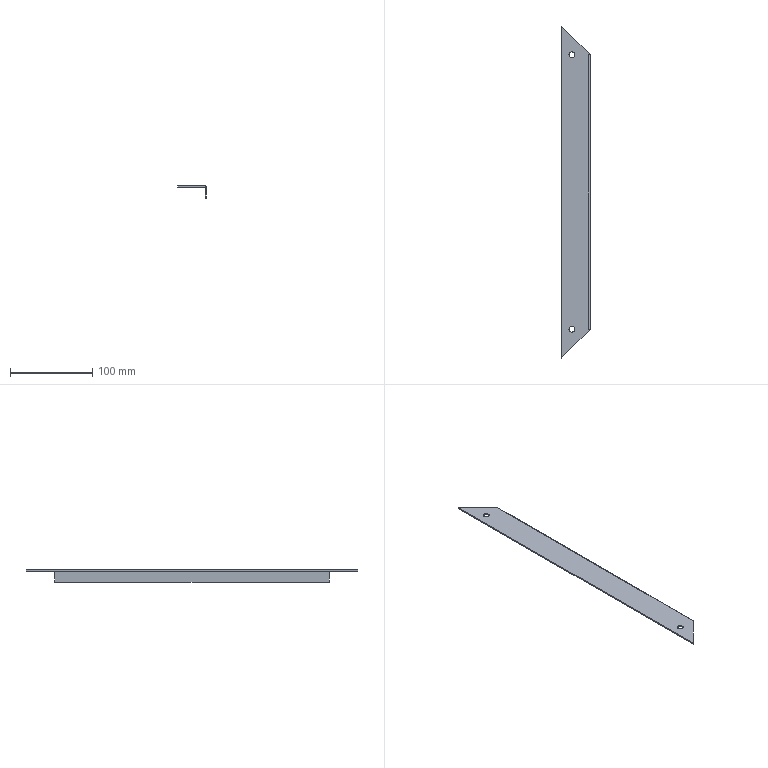Part | STEP file | Right Small Door Clamp Frame 2 | 1 solid | 22 faces | box 35 x 403 x 15 mm | volume 25676 mm3 | plane 14 | cylinder 8 | commonest cylinder face diameters 7 x4 0.15 x2 1 x1 4 x1
STEP:
#1=CARTESIAN_POINT('',(-157.,-97.848,15.));
#2=VERTEX_POINT('',#1);
#3=CARTESIAN_POINT('',(-164.,-97.848,15.));
#4=VERTEX_POINT('',#3);
#5=CARTESIAN_POINT('',(-160.5,-97.848,15.));
#6=DIRECTION('',(0.,0.,-1.));
#7=DIRECTION('',(-1.,0.,0.));
#8=AXIS2_PLACEMENT_3D('',#5,#6,#7);
#9=CIRCLE('',#8,3.5);
#10=EDGE_CURVE('',#2,#4,#9,.T.);
#11=ORIENTED_EDGE('',*,*,#10,.F.);
#12=CARTESIAN_POINT('',(-157.,-97.848,13.5));
#13=VERTEX_POINT('',#12);
#14=CARTESIAN_POINT('',(-157.,-97.848,15.));
#15=DIRECTION('',(0.,0.,-1.));
#16=VECTOR('',#15,1000.);
#17=LINE('',#14,#16);
#18=EDGE_CURVE('',#2,#13,#17,.T.);
#19=ORIENTED_EDGE('',*,*,#18,.T.);
#20=CARTESIAN_POINT('',(-164.,-97.848,13.5));
#21=VERTEX_POINT('',#20);
#22=CARTESIAN_POINT('',(-160.5,-97.848,13.5));
#23=DIRECTION('',(0.,0.,1.));
#24=DIRECTION('',(-1.,0.,0.));
#25=AXIS2_PLACEMENT_3D('',#22,#23,#24);
#26=CIRCLE('',#25,3.5);
#27=EDGE_CURVE('',#21,#13,#26,.T.);
#28=ORIENTED_EDGE('',*,*,#27,.F.);
#29=CARTESIAN_POINT('',(-164.,-97.848,15.));
#30=DIRECTION('',(0.,0.,-1.));
#31=VECTOR('',#30,1000.);
#32=LINE('',#29,#31);
#33=EDGE_CURVE('',#4,#21,#32,.T.);
#34=ORIENTED_EDGE('',*,*,#33,.F.);
#35=EDGE_LOOP('',(#11,#19,#28,#34));
#36=FACE_OUTER_BOUND('',#35,.T.);
#37=CARTESIAN_POINT('',(-160.5,-97.848,15.));
#38=DIRECTION('',(0.,0.,-1.));
#39=DIRECTION('',(-1.,0.,0.));
#40=AXIS2_PLACEMENT_3D('',#37,#38,#39);
#41=CYLINDRICAL_SURFACE('',#40,3.5);
#42=ADVANCED_FACE('',(#36),#41,.F.);
#43=CARTESIAN_POINT('',(-157.,235.152,15.));
#44=VERTEX_POINT('',#43);
#45=CARTESIAN_POINT('',(-164.,235.152,15.));
#46=VERTEX_POINT('',#45);
#47=CARTESIAN_POINT('',(-160.5,235.152,15.));
#48=DIRECTION('',(0.,0.,-1.));
#49=DIRECTION('',(-1.,0.,0.));
#50=AXIS2_PLACEMENT_3D('',#47,#48,#49);
#51=CIRCLE('',#50,3.5);
#52=EDGE_CURVE('',#44,#46,#51,.T.);
#53=ORIENTED_EDGE('',*,*,#52,.F.);
#54=CARTESIAN_POINT('',(-157.,235.152,13.5));
#55=VERTEX_POINT('',#54);
#56=CARTESIAN_POINT('',(-157.,235.152,15.));
#57=DIRECTION('',(0.,0.,-1.));
#58=VECTOR('',#57,1000.);
#59=LINE('',#56,#58);
#60=EDGE_CURVE('',#44,#55,#59,.T.);
#61=ORIENTED_EDGE('',*,*,#60,.T.);
#62=CARTESIAN_POINT('',(-164.,235.152,13.5));
#63=VERTEX_POINT('',#62);
#64=CARTESIAN_POINT('',(-160.5,235.152,13.5));
#65=DIRECTION('',(0.,0.,1.));
#66=DIRECTION('',(-1.,0.,0.));
#67=AXIS2_PLACEMENT_3D('',#64,#65,#66);
#68=CIRCLE('',#67,3.5);
#69=EDGE_CURVE('',#63,#55,#68,.T.);
#70=ORIENTED_EDGE('',*,*,#69,.F.);
#71=CARTESIAN_POINT('',(-164.,235.152,15.));
#72=DIRECTION('',(0.,0.,-1.));
#73=VECTOR('',#72,1000.);
#74=LINE('',#71,#73);
#75=EDGE_CURVE('',#46,#63,#74,.T.);
#76=ORIENTED_EDGE('',*,*,#75,.F.);
#77=EDGE_LOOP('',(#53,#61,#70,#76));
#78=FACE_OUTER_BOUND('',#77,.T.);
#79=CARTESIAN_POINT('',(-160.5,235.152,15.));
#80=DIRECTION('',(0.,0.,-1.));
#81=DIRECTION('',(-1.,0.,0.));
#82=AXIS2_PLACEMENT_3D('',#79,#80,#81);
#83=CYLINDRICAL_SURFACE('',#82,3.5);
#84=ADVANCED_FACE('',(#78),#83,.F.);
#85=CARTESIAN_POINT('',(-140.15,-97.998,15.));
#86=VERTEX_POINT('',#85);
#87=CARTESIAN_POINT('',(-139.5,-97.998,15.));
#88=VERTEX_POINT('',#87);
#89=CARTESIAN_POINT('',(0.,-97.998,15.));
#90=DIRECTION('',(1.,0.,0.));
#91=VECTOR('',#90,1000.);
#92=LINE('',#89,#91);
#93=EDGE_CURVE('',#86,#88,#92,.T.);
#94=ORIENTED_EDGE('',*,*,#93,.F.);
#95=CARTESIAN_POINT('',(-140.15,-97.848,15.));
#96=VERTEX_POINT('',#95);
#97=CARTESIAN_POINT('',(-140.15,-97.923,15.));
#98=DIRECTION('',(0.,0.,-1.));
#99=DIRECTION('',(1.,0.,0.));
#100=AXIS2_PLACEMENT_3D('',#97,#98,#99);
#101=CIRCLE('',#100,0.075);
#102=EDGE_CURVE('',#86,#96,#101,.T.);
#103=ORIENTED_EDGE('',*,*,#102,.T.);
#104=CARTESIAN_POINT('',(-140.,-97.848,15.));
#105=VERTEX_POINT('',#104);
#106=CARTESIAN_POINT('',(0.,-97.848,15.));
#107=DIRECTION('',(-1.,0.,0.));
#108=VECTOR('',#107,1000.);
#109=LINE('',#106,#108);
#110=EDGE_CURVE('',#105,#96,#109,.T.);
#111=ORIENTED_EDGE('',*,*,#110,.F.);
#112=CARTESIAN_POINT('',(-140.,235.152,15.));
#113=VERTEX_POINT('',#112);
#114=CARTESIAN_POINT('',(-140.,0.,15.));
#115=DIRECTION('',(0.,1.,0.));
#116=VECTOR('',#115,1000.);
#117=LINE('',#114,#116);
#118=EDGE_CURVE('',#105,#113,#117,.T.);
#119=ORIENTED_EDGE('',*,*,#118,.T.);
#120=CARTESIAN_POINT('',(-140.15,235.152,15.));
#121=VERTEX_POINT('',#120);
#122=CARTESIAN_POINT('',(0.,235.152,15.));
#123=DIRECTION('',(1.,0.,0.));
#124=VECTOR('',#123,1000.);
#125=LINE('',#122,#124);
#126=EDGE_CURVE('',#121,#113,#125,.T.);
#127=ORIENTED_EDGE('',*,*,#126,.F.);
#128=CARTESIAN_POINT('',(-140.15,235.302,15.));
#129=VERTEX_POINT('',#128);
#130=CARTESIAN_POINT('',(-140.15,235.227,15.));
#131=DIRECTION('',(0.,0.,-1.));
#132=DIRECTION('',(1.,0.,0.));
#133=AXIS2_PLACEMENT_3D('',#130,#131,#132);
#134=CIRCLE('',#133,0.075);
#135=EDGE_CURVE('',#121,#129,#134,.T.);
#136=ORIENTED_EDGE('',*,*,#135,.T.);
#137=CARTESIAN_POINT('',(-139.5,235.302,15.));
#138=VERTEX_POINT('',#137);
#139=CARTESIAN_POINT('',(0.,235.302,15.));
#140=DIRECTION('',(-1.,0.,0.));
#141=VECTOR('',#140,1000.);
#142=LINE('',#139,#141);
#143=EDGE_CURVE('',#138,#129,#142,.T.);
#144=ORIENTED_EDGE('',*,*,#143,.F.);
#145=CARTESIAN_POINT('',(-139.5,236.652,15.));
#146=VERTEX_POINT('',#145);
#147=CARTESIAN_POINT('',(-139.5,0.,15.));
#148=DIRECTION('',(0.,1.,0.));
#149=VECTOR('',#148,1000.);
#150=LINE('',#147,#149);
#151=EDGE_CURVE('',#138,#146,#150,.T.);
#152=ORIENTED_EDGE('',*,*,#151,.T.);
#153=CARTESIAN_POINT('',(-173.,270.152,15.));
#154=VERTEX_POINT('',#153);
#155=CARTESIAN_POINT('',(-139.5,236.652,15.));
#156=DIRECTION('',(-0.7071,0.7071,0.));
#157=VECTOR('',#156,1000.);
#158=LINE('',#155,#157);
#159=EDGE_CURVE('',#146,#154,#158,.T.);
#160=ORIENTED_EDGE('',*,*,#159,.T.);
#161=CARTESIAN_POINT('',(-173.,-132.848,15.));
#162=VERTEX_POINT('',#161);
#163=CARTESIAN_POINT('',(-173.,0.,15.));
#164=DIRECTION('',(0.,-1.,0.));
#165=VECTOR('',#164,1000.);
#166=LINE('',#163,#165);
#167=EDGE_CURVE('',#154,#162,#166,.T.);
#168=ORIENTED_EDGE('',*,*,#167,.T.);
#169=CARTESIAN_POINT('',(-139.5,-99.348,15.));
#170=VERTEX_POINT('',#169);
#171=CARTESIAN_POINT('',(-173.,-132.848,15.));
#172=DIRECTION('',(0.7071,0.7071,0.));
#173=VECTOR('',#172,1000.);
#174=LINE('',#171,#173);
#175=EDGE_CURVE('',#162,#170,#174,.T.);
#176=ORIENTED_EDGE('',*,*,#175,.T.);
#177=CARTESIAN_POINT('',(-139.5,0.,15.));
#178=DIRECTION('',(0.,1.,0.));
#179=VECTOR('',#178,1000.);
#180=LINE('',#177,#179);
#181=EDGE_CURVE('',#170,#88,#180,.T.);
#182=ORIENTED_EDGE('',*,*,#181,.T.);
#183=EDGE_LOOP('',(#94,#103,#111,#119,#127,#136,#144,#152,#160,#168,#176,#182));
#184=FACE_OUTER_BOUND('',#183,.T.);
#185=CARTESIAN_POINT('',(-160.5,-97.848,15.));
#186=DIRECTION('',(0.,0.,-1.));
#187=DIRECTION('',(-1.,0.,0.));
#188=AXIS2_PLACEMENT_3D('',#185,#186,#187);
#189=CIRCLE('',#188,3.5);
#190=EDGE_CURVE('',#4,#2,#189,.T.);
#191=ORIENTED_EDGE('',*,*,#190,.T.);
#192=ORIENTED_EDGE('',*,*,#10,.T.);
#193=EDGE_LOOP('',(#191,#192));
#194=FACE_BOUND('',#193,.T.);
#195=CARTESIAN_POINT('',(-160.5,235.152,15.));
#196=DIRECTION('',(0.,0.,-1.));
#197=DIRECTION('',(-1.,0.,0.));
#198=AXIS2_PLACEMENT_3D('',#195,#196,#197);
#199=CIRCLE('',#198,3.5);
#200=EDGE_CURVE('',#46,#44,#199,.T.);
#201=ORIENTED_EDGE('',*,*,#200,.T.);
#202=ORIENTED_EDGE('',*,*,#52,.T.);
#203=EDGE_LOOP('',(#201,#202));
#204=FACE_BOUND('',#203,.T.);
#205=CARTESIAN_POINT('',(0.,0.,15.));
#206=DIRECTION('',(0.,0.,1.));
#207=DIRECTION('',(1.,0.,0.));
#208=AXIS2_PLACEMENT_3D('',#205,#206,#207);
#209=PLANE('',#208);
#210=ADVANCED_FACE('',(#184,#194,#204),#209,.T.);
#211=CARTESIAN_POINT('',(-139.5,-99.348,13.5));
#212=VERTEX_POINT('',#211);
#213=CARTESIAN_POINT('',(-139.5,-99.348,-793.78));
#214=DIRECTION('',(0.,0.,-1.));
#215=VECTOR('',#214,1000.);
#216=LINE('',#213,#215);
#217=EDGE_CURVE('',#170,#212,#216,.T.);
#218=ORIENTED_EDGE('',*,*,#217,.T.);
#219=CARTESIAN_POINT('',(-139.5,-97.998,13.5));
#220=VERTEX_POINT('',#219);
#221=CARTESIAN_POINT('',(-139.5,0.,13.5));
#222=DIRECTION('',(0.,1.,0.));
#223=VECTOR('',#222,1000.);
#224=LINE('',#221,#223);
#225=EDGE_CURVE('',#212,#220,#224,.T.);
#226=ORIENTED_EDGE('',*,*,#225,.T.);
#227=CARTESIAN_POINT('',(-139.5,-97.998,-793.78));
#228=DIRECTION('',(0.,0.,1.));
#229=VECTOR('',#228,1000.);
#230=LINE('',#227,#229);
#231=EDGE_CURVE('',#220,#88,#230,.T.);
#232=ORIENTED_EDGE('',*,*,#231,.T.);
#233=ORIENTED_EDGE('',*,*,#181,.F.);
#234=EDGE_LOOP('',(#218,#226,#232,#233));
#235=FACE_OUTER_BOUND('',#234,.T.);
#236=CARTESIAN_POINT('',(-139.5,0.,-793.78));
#237=DIRECTION('',(1.,0.,0.));
#238=DIRECTION('',(0.,1.,0.));
#239=AXIS2_PLACEMENT_3D('',#236,#237,#238);
#240=PLANE('',#239);
#241=ADVANCED_FACE('',(#235),#240,.T.);
#242=CARTESIAN_POINT('',(-173.,-132.848,13.5));
#243=VERTEX_POINT('',#242);
#244=CARTESIAN_POINT('',(-173.,-132.848,-793.78));
#245=DIRECTION('',(0.,0.,-1.));
#246=VECTOR('',#245,1000.);
#247=LINE('',#244,#246);
#248=EDGE_CURVE('',#162,#243,#247,.T.);
#249=ORIENTED_EDGE('',*,*,#248,.T.);
#250=CARTESIAN_POINT('',(-20.076,20.076,13.5));
#251=DIRECTION('',(0.7071,0.7071,0.));
#252=VECTOR('',#251,1000.);
#253=LINE('',#250,#252);
#254=EDGE_CURVE('',#243,#212,#253,.T.);
#255=ORIENTED_EDGE('',*,*,#254,.T.);
#256=ORIENTED_EDGE('',*,*,#217,.F.);
#257=ORIENTED_EDGE('',*,*,#175,.F.);
#258=EDGE_LOOP('',(#249,#255,#256,#257));
#259=FACE_OUTER_BOUND('',#258,.T.);
#260=CARTESIAN_POINT('',(-20.076,20.076,-793.78));
#261=DIRECTION('',(0.7071,-0.7071,0.));
#262=DIRECTION('',(0.7071,0.7071,0.));
#263=AXIS2_PLACEMENT_3D('',#260,#261,#262);
#264=PLANE('',#263);
#265=ADVANCED_FACE('',(#259),#264,.T.);
#266=CARTESIAN_POINT('',(-173.,270.152,13.5));
#267=VERTEX_POINT('',#266);
#268=CARTESIAN_POINT('',(-173.,270.152,-793.78));
#269=DIRECTION('',(0.,0.,-1.));
#270=VECTOR('',#269,1000.);
#271=LINE('',#268,#270);
#272=EDGE_CURVE('',#154,#267,#271,.T.);
#273=ORIENTED_EDGE('',*,*,#272,.T.);
#274=CARTESIAN_POINT('',(-173.,270.152,13.5));
#275=DIRECTION('',(0.,-1.,0.));
#276=VECTOR('',#275,1000.);
#277=LINE('',#274,#276);
#278=EDGE_CURVE('',#267,#243,#277,.T.);
#279=ORIENTED_EDGE('',*,*,#278,.T.);
#280=ORIENTED_EDGE('',*,*,#248,.F.);
#281=ORIENTED_EDGE('',*,*,#167,.F.);
#282=EDGE_LOOP('',(#273,#279,#280,#281));
#283=FACE_OUTER_BOUND('',#282,.T.);
#284=CARTESIAN_POINT('',(-173.,270.152,-793.78));
#285=DIRECTION('',(-1.,0.,0.));
#286=DIRECTION('',(0.,0.,1.));
#287=AXIS2_PLACEMENT_3D('',#284,#285,#286);
#288=PLANE('',#287);
#289=ADVANCED_FACE('',(#283),#288,.T.);
#290=CARTESIAN_POINT('',(-139.5,236.652,13.5));
#291=VERTEX_POINT('',#290);
#292=CARTESIAN_POINT('',(-139.5,236.652,-793.78));
#293=DIRECTION('',(0.,0.,-1.));
#294=VECTOR('',#293,1000.);
#295=LINE('',#292,#294);
#296=EDGE_CURVE('',#146,#291,#295,.T.);
#297=ORIENTED_EDGE('',*,*,#296,.T.);
#298=CARTESIAN_POINT('',(48.576,48.576,13.5));
#299=DIRECTION('',(-0.7071,0.7071,0.));
#300=VECTOR('',#299,1000.);
#301=LINE('',#298,#300);
#302=EDGE_CURVE('',#291,#267,#301,.T.);
#303=ORIENTED_EDGE('',*,*,#302,.T.);
#304=ORIENTED_EDGE('',*,*,#272,.F.);
#305=ORIENTED_EDGE('',*,*,#159,.F.);
#306=EDGE_LOOP('',(#297,#303,#304,#305));
#307=FACE_OUTER_BOUND('',#306,.T.);
#308=CARTESIAN_POINT('',(48.576,48.576,-793.78));
#309=DIRECTION('',(0.7071,0.7071,0.));
#310=DIRECTION('',(-0.7071,0.7071,0.));
#311=AXIS2_PLACEMENT_3D('',#308,#309,#310);
#312=PLANE('',#311);
#313=ADVANCED_FACE('',(#307),#312,.T.);
#314=CARTESIAN_POINT('',(-139.5,235.302,13.5));
#315=VERTEX_POINT('',#314);
#316=CARTESIAN_POINT('',(-139.5,235.302,-793.78));
#317=DIRECTION('',(0.,0.,1.));
#318=VECTOR('',#317,1000.);
#319=LINE('',#316,#318);
#320=EDGE_CURVE('',#315,#138,#319,.T.);
#321=ORIENTED_EDGE('',*,*,#320,.F.);
#322=CARTESIAN_POINT('',(-139.5,235.152,13.5));
#323=DIRECTION('',(0.,-1.,0.));
#324=VECTOR('',#323,1000.);
#325=LINE('',#322,#324);
#326=EDGE_CURVE('',#291,#315,#325,.T.);
#327=ORIENTED_EDGE('',*,*,#326,.F.);
#328=ORIENTED_EDGE('',*,*,#296,.F.);
#329=ORIENTED_EDGE('',*,*,#151,.F.);
#330=EDGE_LOOP('',(#321,#327,#328,#329));
#331=FACE_OUTER_BOUND('',#330,.T.);
#332=CARTESIAN_POINT('',(-139.5,235.152,-793.78));
#333=DIRECTION('',(-1.,0.,0.));
#334=DIRECTION('',(0.,-1.,0.));
#335=AXIS2_PLACEMENT_3D('',#332,#333,#334);
#336=PLANE('',#335);
#337=ADVANCED_FACE('',(#331),#336,.F.);
#338=CARTESIAN_POINT('',(-138.,-97.848,13.));
#339=VERTEX_POINT('',#338);
#340=CARTESIAN_POINT('',(-138.,235.152,13.));
#341=VERTEX_POINT('',#340);
#342=CARTESIAN_POINT('',(-138.,640.963,13.));
#343=DIRECTION('',(0.,1.,0.));
#344=VECTOR('',#343,1000.);
#345=LINE('',#342,#344);
#346=EDGE_CURVE('',#339,#341,#345,.T.);
#347=ORIENTED_EDGE('',*,*,#346,.T.);
#348=CARTESIAN_POINT('',(-140.,235.152,13.));
#349=DIRECTION('',(0.,-1.,0.));
#350=DIRECTION('',(0.,0.,-1.));
#351=AXIS2_PLACEMENT_3D('',#348,#349,#350);
#352=CIRCLE('',#351,2.);
#353=EDGE_CURVE('',#341,#113,#352,.T.);
#354=ORIENTED_EDGE('',*,*,#353,.T.);
#355=ORIENTED_EDGE('',*,*,#118,.F.);
#356=CARTESIAN_POINT('',(-140.,-97.848,13.));
#357=DIRECTION('',(0.,1.,0.));
#358=DIRECTION('',(0.,0.,-1.));
#359=AXIS2_PLACEMENT_3D('',#356,#357,#358);
#360=CIRCLE('',#359,2.);
#361=EDGE_CURVE('',#105,#339,#360,.T.);
#362=ORIENTED_EDGE('',*,*,#361,.T.);
#363=EDGE_LOOP('',(#347,#354,#355,#362));
#364=FACE_OUTER_BOUND('',#363,.T.);
#365=CARTESIAN_POINT('',(-140.,640.963,13.));
#366=DIRECTION('',(0.,-1.,0.));
#367=DIRECTION('',(0.,0.,-1.));
#368=AXIS2_PLACEMENT_3D('',#365,#366,#367);
#369=CYLINDRICAL_SURFACE('',#368,2.);
#370=ADVANCED_FACE('',(#364),#369,.T.);
#371=ORIENTED_EDGE('',*,*,#18,.F.);
#372=ORIENTED_EDGE('',*,*,#190,.F.);
#373=ORIENTED_EDGE('',*,*,#33,.T.);
#374=CARTESIAN_POINT('',(-160.5,-97.848,13.5));
#375=DIRECTION('',(0.,0.,1.));
#376=DIRECTION('',(-1.,0.,0.));
#377=AXIS2_PLACEMENT_3D('',#374,#375,#376);
#378=CIRCLE('',#377,3.5);
#379=EDGE_CURVE('',#13,#21,#378,.T.);
#380=ORIENTED_EDGE('',*,*,#379,.F.);
#381=EDGE_LOOP('',(#371,#372,#373,#380));
#382=FACE_OUTER_BOUND('',#381,.T.);
#383=CARTESIAN_POINT('',(-160.5,-97.848,15.));
#384=DIRECTION('',(0.,0.,-1.));
#385=DIRECTION('',(-1.,0.,0.));
#386=AXIS2_PLACEMENT_3D('',#383,#384,#385);
#387=CYLINDRICAL_SURFACE('',#386,3.5);
#388=ADVANCED_FACE('',(#382),#387,.F.);
#389=ORIENTED_EDGE('',*,*,#60,.F.);
#390=ORIENTED_EDGE('',*,*,#200,.F.);
#391=ORIENTED_EDGE('',*,*,#75,.T.);
#392=CARTESIAN_POINT('',(-160.5,235.152,13.5));
#393=DIRECTION('',(0.,0.,1.));
#394=DIRECTION('',(-1.,0.,0.));
#395=AXIS2_PLACEMENT_3D('',#392,#393,#394);
#396=CIRCLE('',#395,3.5);
#397=EDGE_CURVE('',#55,#63,#396,.T.);
#398=ORIENTED_EDGE('',*,*,#397,.F.);
#399=EDGE_LOOP('',(#389,#390,#391,#398));
#400=FACE_OUTER_BOUND('',#399,.T.);
#401=CARTESIAN_POINT('',(-160.5,235.152,15.));
#402=DIRECTION('',(0.,0.,-1.));
#403=DIRECTION('',(-1.,0.,0.));
#404=AXIS2_PLACEMENT_3D('',#401,#402,#403);
#405=CYLINDRICAL_SURFACE('',#404,3.5);
#406=ADVANCED_FACE('',(#400),#405,.F.);
#407=ORIENTED_EDGE('',*,*,#231,.F.);
#408=CARTESIAN_POINT('',(-140.15,-97.998,13.5));
#409=VERTEX_POINT('',#408);
#410=CARTESIAN_POINT('',(0.,-97.998,13.5));
#411=DIRECTION('',(-1.,0.,0.));
#412=VECTOR('',#411,1000.);
#413=LINE('',#410,#412);
#414=EDGE_CURVE('',#220,#409,#413,.T.);
#415=ORIENTED_EDGE('',*,*,#414,.T.);
#416=CARTESIAN_POINT('',(-140.15,-97.998,-793.78));
#417=DIRECTION('',(0.,0.,1.));
#418=VECTOR('',#417,1000.);
#419=LINE('',#416,#418);
#420=EDGE_CURVE('',#409,#86,#419,.T.);
#421=ORIENTED_EDGE('',*,*,#420,.T.);
#422=ORIENTED_EDGE('',*,*,#93,.T.);
#423=EDGE_LOOP('',(#407,#415,#421,#422));
#424=FACE_OUTER_BOUND('',#423,.T.);
#425=CARTESIAN_POINT('',(0.,-97.998,-793.78));
#426=DIRECTION('',(0.,1.,0.));
#427=DIRECTION('',(0.,0.,1.));
#428=AXIS2_PLACEMENT_3D('',#425,#426,#427);
#429=PLANE('',#428);
#430=ADVANCED_FACE('',(#424),#429,.T.);
#431=CARTESIAN_POINT('',(-140.15,-97.848,13.5));
#432=VERTEX_POINT('',#431);
#433=CARTESIAN_POINT('',(-140.,-97.848,13.5));
#434=VERTEX_POINT('',#433);
#435=CARTESIAN_POINT('',(0.,-97.848,13.5));
#436=DIRECTION('',(1.,0.,0.));
#437=VECTOR('',#436,1000.);
#438=LINE('',#435,#437);
#439=EDGE_CURVE('',#432,#434,#438,.T.);
#440=ORIENTED_EDGE('',*,*,#439,.F.);
#441=CARTESIAN_POINT('',(-140.15,-97.923,13.5));
#442=DIRECTION('',(0.,0.,-1.));
#443=DIRECTION('',(1.,0.,0.));
#444=AXIS2_PLACEMENT_3D('',#441,#442,#443);
#445=CIRCLE('',#444,0.075);
#446=EDGE_CURVE('',#409,#432,#445,.T.);
#447=ORIENTED_EDGE('',*,*,#446,.F.);
#448=ORIENTED_EDGE('',*,*,#414,.F.);
#449=ORIENTED_EDGE('',*,*,#225,.F.);
#450=ORIENTED_EDGE('',*,*,#254,.F.);
#451=ORIENTED_EDGE('',*,*,#278,.F.);
#452=ORIENTED_EDGE('',*,*,#302,.F.);
#453=ORIENTED_EDGE('',*,*,#326,.T.);
#454=CARTESIAN_POINT('',(-140.15,235.302,13.5));
#455=VERTEX_POINT('',#454);
#456=CARTESIAN_POINT('',(0.,235.302,13.5));
#457=DIRECTION('',(1.,0.,0.));
#458=VECTOR('',#457,1000.);
#459=LINE('',#456,#458);
#460=EDGE_CURVE('',#455,#315,#459,.T.);
#461=ORIENTED_EDGE('',*,*,#460,.F.);
#462=CARTESIAN_POINT('',(-140.15,235.152,13.5));
#463=VERTEX_POINT('',#462);
#464=CARTESIAN_POINT('',(-140.15,235.227,13.5));
#465=DIRECTION('',(0.,0.,1.));
#466=DIRECTION('',(1.,0.,0.));
#467=AXIS2_PLACEMENT_3D('',#464,#465,#466);
#468=CIRCLE('',#467,0.075);
#469=EDGE_CURVE('',#455,#463,#468,.T.);
#470=ORIENTED_EDGE('',*,*,#469,.T.);
#471=CARTESIAN_POINT('',(-140.,235.152,13.5));
#472=VERTEX_POINT('',#471);
#473=CARTESIAN_POINT('',(0.,235.152,13.5));
#474=DIRECTION('',(-1.,0.,0.));
#475=VECTOR('',#474,1000.);
#476=LINE('',#473,#475);
#477=EDGE_CURVE('',#472,#463,#476,.T.);
#478=ORIENTED_EDGE('',*,*,#477,.F.);
#479=CARTESIAN_POINT('',(-140.,0.,13.5));
#480=DIRECTION('',(0.,1.,0.));
#481=VECTOR('',#480,1000.);
#482=LINE('',#479,#481);
#483=EDGE_CURVE('',#434,#472,#482,.T.);
#484=ORIENTED_EDGE('',*,*,#483,.F.);
#485=EDGE_LOOP('',(#440,#447,#448,#449,#450,#451,#452,#453,#461,#470,#478,#484));
#486=FACE_OUTER_BOUND('',#485,.T.);
#487=ORIENTED_EDGE('',*,*,#27,.T.);
#488=ORIENTED_EDGE('',*,*,#379,.T.);
#489=EDGE_LOOP('',(#487,#488));
#490=FACE_BOUND('',#489,.T.);
#491=ORIENTED_EDGE('',*,*,#69,.T.);
#492=ORIENTED_EDGE('',*,*,#397,.T.);
#493=EDGE_LOOP('',(#491,#492));
#494=FACE_BOUND('',#493,.T.);
#495=CARTESIAN_POINT('',(0.,0.,13.5));
#496=DIRECTION('',(0.,0.,1.));
#497=DIRECTION('',(1.,0.,0.));
#498=AXIS2_PLACEMENT_3D('',#495,#496,#497);
#499=PLANE('',#498);
#500=ADVANCED_FACE('',(#486,#490,#494),#499,.F.);
#501=CARTESIAN_POINT('',(-140.15,235.302,-793.78));
#502=DIRECTION('',(0.,0.,-1.));
#503=VECTOR('',#502,1000.);
#504=LINE('',#501,#503);
#505=EDGE_CURVE('',#129,#455,#504,.T.);
#506=ORIENTED_EDGE('',*,*,#505,.T.);
#507=ORIENTED_EDGE('',*,*,#460,.T.);
#508=ORIENTED_EDGE('',*,*,#320,.T.);
#509=ORIENTED_EDGE('',*,*,#143,.T.);
#510=EDGE_LOOP('',(#506,#507,#508,#509));
#511=FACE_OUTER_BOUND('',#510,.T.);
#512=CARTESIAN_POINT('',(0.,235.302,-793.78));
#513=DIRECTION('',(0.,-1.,0.));
#514=DIRECTION('',(0.,0.,-1.));
#515=AXIS2_PLACEMENT_3D('',#512,#513,#514);
#516=PLANE('',#515);
#517=ADVANCED_FACE('',(#511),#516,.T.);
#518=CARTESIAN_POINT('',(-139.5,235.152,13.));
#519=VERTEX_POINT('',#518);
#520=CARTESIAN_POINT('',(-140.,235.152,13.));
#521=DIRECTION('',(0.,-1.,0.));
#522=DIRECTION('',(0.,0.,-1.));
#523=AXIS2_PLACEMENT_3D('',#520,#521,#522);
#524=CIRCLE('',#523,0.5);
#525=EDGE_CURVE('',#519,#472,#524,.T.);
#526=ORIENTED_EDGE('',*,*,#525,.T.);
#527=ORIENTED_EDGE('',*,*,#477,.T.);
#528=CARTESIAN_POINT('',(-140.15,235.152,-793.78));
#529=DIRECTION('',(0.,0.,1.));
#530=VECTOR('',#529,1000.);
#531=LINE('',#528,#530);
#532=EDGE_CURVE('',#463,#121,#531,.T.);
#533=ORIENTED_EDGE('',*,*,#532,.T.);
#534=ORIENTED_EDGE('',*,*,#126,.T.);
#535=ORIENTED_EDGE('',*,*,#353,.F.);
#536=CARTESIAN_POINT('',(-138.,235.152,0.));
#537=VERTEX_POINT('',#536);
#538=CARTESIAN_POINT('',(-138.,235.152,15.));
#539=DIRECTION('',(0.,0.,1.));
#540=VECTOR('',#539,1000.);
#541=LINE('',#538,#540);
#542=EDGE_CURVE('',#537,#341,#541,.T.);
#543=ORIENTED_EDGE('',*,*,#542,.F.);
#544=CARTESIAN_POINT('',(-139.5,235.152,0.));
#545=VERTEX_POINT('',#544);
#546=CARTESIAN_POINT('',(-804.507,235.152,0.));
#547=DIRECTION('',(-1.,0.,0.));
#548=VECTOR('',#547,1000.);
#549=LINE('',#546,#548);
#550=EDGE_CURVE('',#537,#545,#549,.T.);
#551=ORIENTED_EDGE('',*,*,#550,.T.);
#552=CARTESIAN_POINT('',(-139.5,235.152,0.));
#553=DIRECTION('',(0.,0.,1.));
#554=VECTOR('',#553,1000.);
#555=LINE('',#552,#554);
#556=EDGE_CURVE('',#545,#519,#555,.T.);
#557=ORIENTED_EDGE('',*,*,#556,.T.);
#558=EDGE_LOOP('',(#526,#527,#533,#534,#535,#543,#551,#557));
#559=FACE_OUTER_BOUND('',#558,.T.);
#560=CARTESIAN_POINT('',(-140.,235.152,13.));
#561=DIRECTION('',(0.,1.,0.));
#562=DIRECTION('',(0.,0.,1.));
#563=AXIS2_PLACEMENT_3D('',#560,#561,#562);
#564=PLANE('',#563);
#565=ADVANCED_FACE('',(#559),#564,.T.);
#566=CARTESIAN_POINT('',(-138.,-97.848,0.));
#567=VERTEX_POINT('',#566);
#568=CARTESIAN_POINT('',(-138.,235.152,0.));
#569=DIRECTION('',(0.,1.,0.));
#570=VECTOR('',#569,1000.);
#571=LINE('',#568,#570);
#572=EDGE_CURVE('',#567,#537,#571,.T.);
#573=ORIENTED_EDGE('',*,*,#572,.T.);
#574=ORIENTED_EDGE('',*,*,#542,.T.);
#575=ORIENTED_EDGE('',*,*,#346,.F.);
#576=CARTESIAN_POINT('',(-138.,-97.848,15.));
#577=DIRECTION('',(0.,0.,-1.));
#578=VECTOR('',#577,1000.);
#579=LINE('',#576,#578);
#580=EDGE_CURVE('',#339,#567,#579,.T.);
#581=ORIENTED_EDGE('',*,*,#580,.T.);
#582=EDGE_LOOP('',(#573,#574,#575,#581));
#583=FACE_OUTER_BOUND('',#582,.T.);
#584=CARTESIAN_POINT('',(-138.,235.152,15.));
#585=DIRECTION('',(1.,0.,0.));
#586=DIRECTION('',(0.,1.,0.));
#587=AXIS2_PLACEMENT_3D('',#584,#585,#586);
#588=PLANE('',#587);
#589=ADVANCED_FACE('',(#583),#588,.T.);
#590=ORIENTED_EDGE('',*,*,#361,.F.);
#591=ORIENTED_EDGE('',*,*,#110,.T.);
#592=CARTESIAN_POINT('',(-140.15,-97.848,-793.78));
#593=DIRECTION('',(0.,0.,-1.));
#594=VECTOR('',#593,1000.);
#595=LINE('',#592,#594);
#596=EDGE_CURVE('',#96,#432,#595,.T.);
#597=ORIENTED_EDGE('',*,*,#596,.T.);
#598=ORIENTED_EDGE('',*,*,#439,.T.);
#599=CARTESIAN_POINT('',(-139.5,-97.848,13.));
#600=VERTEX_POINT('',#599);
#601=CARTESIAN_POINT('',(-140.,-97.848,13.));
#602=DIRECTION('',(0.,1.,0.));
#603=DIRECTION('',(0.,0.,-1.));
#604=AXIS2_PLACEMENT_3D('',#601,#602,#603);
#605=CIRCLE('',#604,0.5);
#606=EDGE_CURVE('',#434,#600,#605,.T.);
#607=ORIENTED_EDGE('',*,*,#606,.T.);
#608=CARTESIAN_POINT('',(-139.5,-97.848,0.));
#609=VERTEX_POINT('',#608);
#610=CARTESIAN_POINT('',(-139.5,-97.848,0.));
#611=DIRECTION('',(0.,0.,1.));
#612=VECTOR('',#611,1000.);
#613=LINE('',#610,#612);
#614=EDGE_CURVE('',#609,#600,#613,.T.);
#615=ORIENTED_EDGE('',*,*,#614,.F.);
#616=CARTESIAN_POINT('',(-804.507,-97.848,0.));
#617=DIRECTION('',(1.,0.,0.));
#618=VECTOR('',#617,1000.);
#619=LINE('',#616,#618);
#620=EDGE_CURVE('',#609,#567,#619,.T.);
#621=ORIENTED_EDGE('',*,*,#620,.T.);
#622=ORIENTED_EDGE('',*,*,#580,.F.);
#623=EDGE_LOOP('',(#590,#591,#597,#598,#607,#615,#621,#622));
#624=FACE_OUTER_BOUND('',#623,.T.);
#625=CARTESIAN_POINT('',(-140.,-97.848,13.));
#626=DIRECTION('',(0.,-1.,0.));
#627=DIRECTION('',(0.,0.,-1.));
#628=AXIS2_PLACEMENT_3D('',#625,#626,#627);
#629=PLANE('',#628);
#630=ADVANCED_FACE('',(#624),#629,.T.);
#631=ORIENTED_EDGE('',*,*,#420,.F.);
#632=ORIENTED_EDGE('',*,*,#446,.T.);
#633=ORIENTED_EDGE('',*,*,#596,.F.);
#634=ORIENTED_EDGE('',*,*,#102,.F.);
#635=EDGE_LOOP('',(#631,#632,#633,#634));
#636=FACE_OUTER_BOUND('',#635,.T.);
#637=CARTESIAN_POINT('',(-140.15,-97.923,-793.78));
#638=DIRECTION('',(0.,0.,1.));
#639=DIRECTION('',(1.,0.,0.));
#640=AXIS2_PLACEMENT_3D('',#637,#638,#639);
#641=CYLINDRICAL_SURFACE('',#640,0.075);
#642=ADVANCED_FACE('',(#636),#641,.F.);
#643=ORIENTED_EDGE('',*,*,#525,.F.);
#644=CARTESIAN_POINT('',(-139.5,640.963,13.));
#645=DIRECTION('',(0.,1.,0.));
#646=VECTOR('',#645,1000.);
#647=LINE('',#644,#646);
#648=EDGE_CURVE('',#600,#519,#647,.T.);
#649=ORIENTED_EDGE('',*,*,#648,.F.);
#650=ORIENTED_EDGE('',*,*,#606,.F.);
#651=ORIENTED_EDGE('',*,*,#483,.T.);
#652=EDGE_LOOP('',(#643,#649,#650,#651));
#653=FACE_OUTER_BOUND('',#652,.T.);
#654=CARTESIAN_POINT('',(-140.,640.963,13.));
#655=DIRECTION('',(0.,-1.,0.));
#656=DIRECTION('',(0.,0.,-1.));
#657=AXIS2_PLACEMENT_3D('',#654,#655,#656);
#658=CYLINDRICAL_SURFACE('',#657,0.5);
#659=ADVANCED_FACE('',(#653),#658,.F.);
#660=ORIENTED_EDGE('',*,*,#532,.F.);
#661=ORIENTED_EDGE('',*,*,#469,.F.);
#662=ORIENTED_EDGE('',*,*,#505,.F.);
#663=ORIENTED_EDGE('',*,*,#135,.F.);
#664=EDGE_LOOP('',(#660,#661,#662,#663));
#665=FACE_OUTER_BOUND('',#664,.T.);
#666=CARTESIAN_POINT('',(-140.15,235.227,-793.78));
#667=DIRECTION('',(0.,0.,1.));
#668=DIRECTION('',(1.,0.,0.));
#669=AXIS2_PLACEMENT_3D('',#666,#667,#668);
#670=CYLINDRICAL_SURFACE('',#669,0.075);
#671=ADVANCED_FACE('',(#665),#670,.F.);
#672=ORIENTED_EDGE('',*,*,#620,.F.);
#673=CARTESIAN_POINT('',(-139.5,235.152,0.));
#674=DIRECTION('',(0.,-1.,0.));
#675=VECTOR('',#674,1000.);
#676=LINE('',#673,#675);
#677=EDGE_CURVE('',#545,#609,#676,.T.);
#678=ORIENTED_EDGE('',*,*,#677,.F.);
#679=ORIENTED_EDGE('',*,*,#550,.F.);
#680=ORIENTED_EDGE('',*,*,#572,.F.);
#681=EDGE_LOOP('',(#672,#678,#679,#680));
#682=FACE_OUTER_BOUND('',#681,.T.);
#683=CARTESIAN_POINT('',(-804.507,235.152,0.));
#684=DIRECTION('',(0.,0.,1.));
#685=DIRECTION('',(0.,-1.,0.));
#686=AXIS2_PLACEMENT_3D('',#683,#684,#685);
#687=PLANE('',#686);
#688=ADVANCED_FACE('',(#682),#687,.F.);
#689=ORIENTED_EDGE('',*,*,#648,.T.);
#690=ORIENTED_EDGE('',*,*,#556,.F.);
#691=ORIENTED_EDGE('',*,*,#677,.T.);
#692=ORIENTED_EDGE('',*,*,#614,.T.);
#693=EDGE_LOOP('',(#689,#690,#691,#692));
#694=FACE_OUTER_BOUND('',#693,.T.);
#695=CARTESIAN_POINT('',(-139.5,235.152,15.));
#696=DIRECTION('',(1.,0.,0.));
#697=DIRECTION('',(0.,1.,0.));
#698=AXIS2_PLACEMENT_3D('',#695,#696,#697);
#699=PLANE('',#698);
#700=ADVANCED_FACE('',(#694),#699,.F.);
#701=CLOSED_SHELL('',(#42,#84,#210,#241,#265,#289,#313,#337,#370,#388,#406,#430,#500,#517,#565,#589,#630,#642,#659,#671,#688,#700));
#702=MANIFOLD_SOLID_BREP('',#701);
#703=CARTESIAN_POINT('',(0.,0.,0.));
#704=DIRECTION('',(0.,0.,1.));
#705=DIRECTION('',(1.,0.,0.));
#706=AXIS2_PLACEMENT_3D('',#703,#704,#705);
#707=(LENGTH_UNIT()NAMED_UNIT(*)SI_UNIT(.MILLI.,.METRE.));
#708=UNCERTAINTY_MEASURE_WITH_UNIT(LENGTH_MEASURE(0.00001),#707,'','');
#709=(NAMED_UNIT(*)PLANE_ANGLE_UNIT()SI_UNIT($,.RADIAN.));
#710=(NAMED_UNIT(*)SI_UNIT($,.STERADIAN.)SOLID_ANGLE_UNIT());
#711=(GEOMETRIC_REPRESENTATION_CONTEXT(3)GLOBAL_UNCERTAINTY_ASSIGNED_CONTEXT((#708))GLOBAL_UNIT_ASSIGNED_CONTEXT((#707,#709,#710))REPRESENTATION_CONTEXT('',''));
#712=ADVANCED_BREP_SHAPE_REPRESENTATION('',(#702,#706),#711);